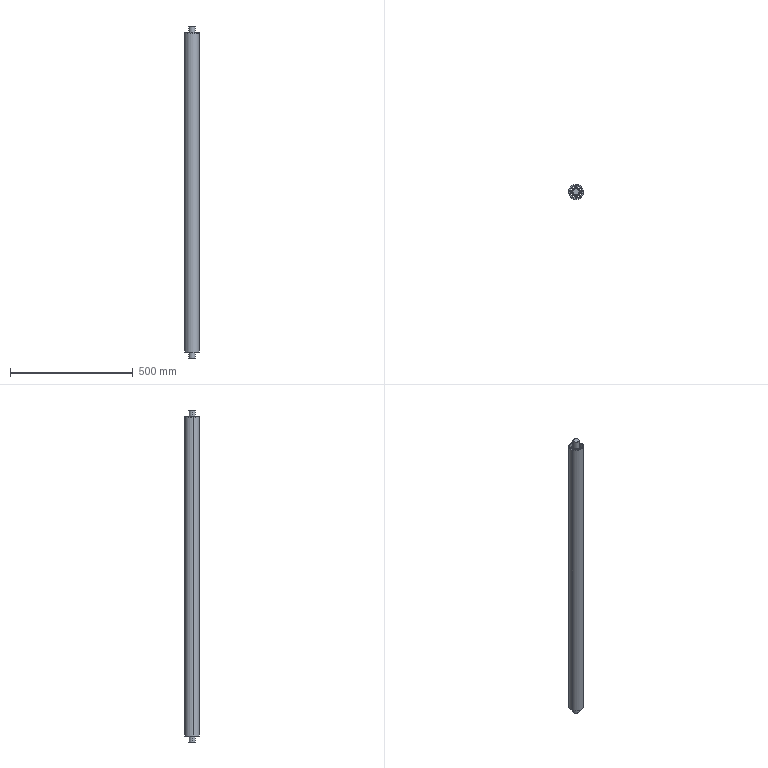Part | SolidWorks | 4 solids | 248 faces | box 60 x 60 x 1352 mm | volume 1988241 mm3 | torus 124 | sphere 68 | cylinder 34 | plane 14 | cone 8 | commonest cylinder face diameters 23 x8 29 x8 17 x4 35 x4 52 x4 25 x2